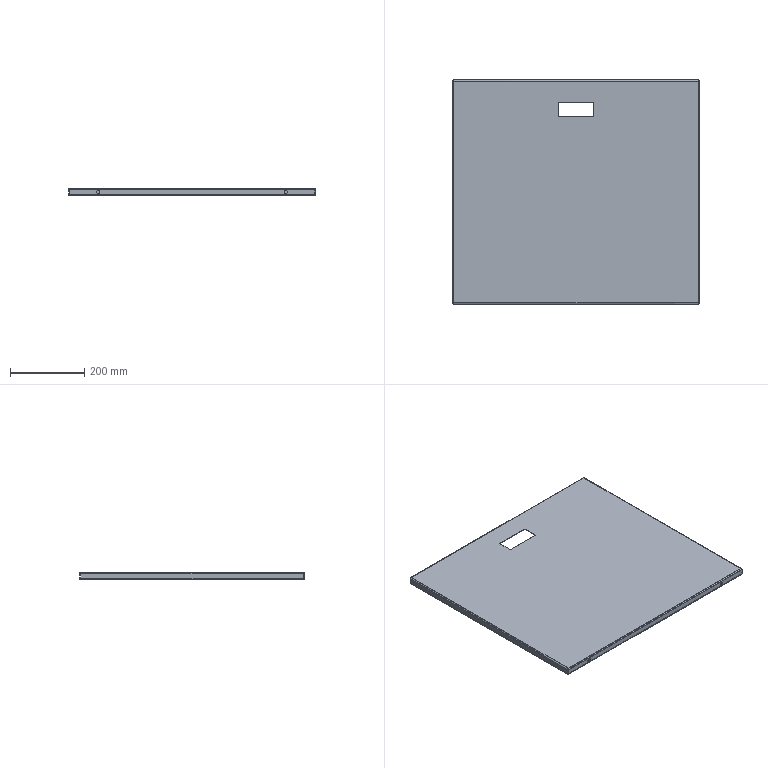Part | SolidWorks | features EdgeFlange 2, FlatPattern 1, HoleWzd 1, SMBaseFlange 1, SheetMetal 1 | 1 solid | 78 faces | box 665 x 605 x 20 mm | volume 726461 mm3 | plane 42 | cylinder 20 | spline 16 | commonest cylinder face diameters 4 x8 7 x8 9 x4